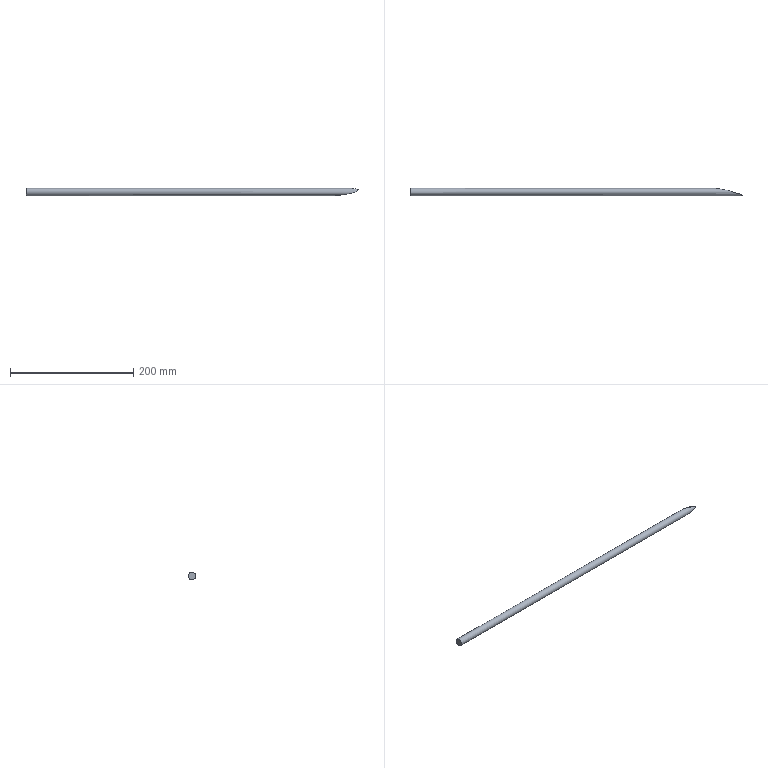Part | STEP file | solid 185 | 1 solid | 4 faces | box 539.477 x 12.005 x 12.001 mm | volume 58014 mm3 | spline 2 | cylinder 1 | plane 1 | commonest cylinder face diameters 12 x1